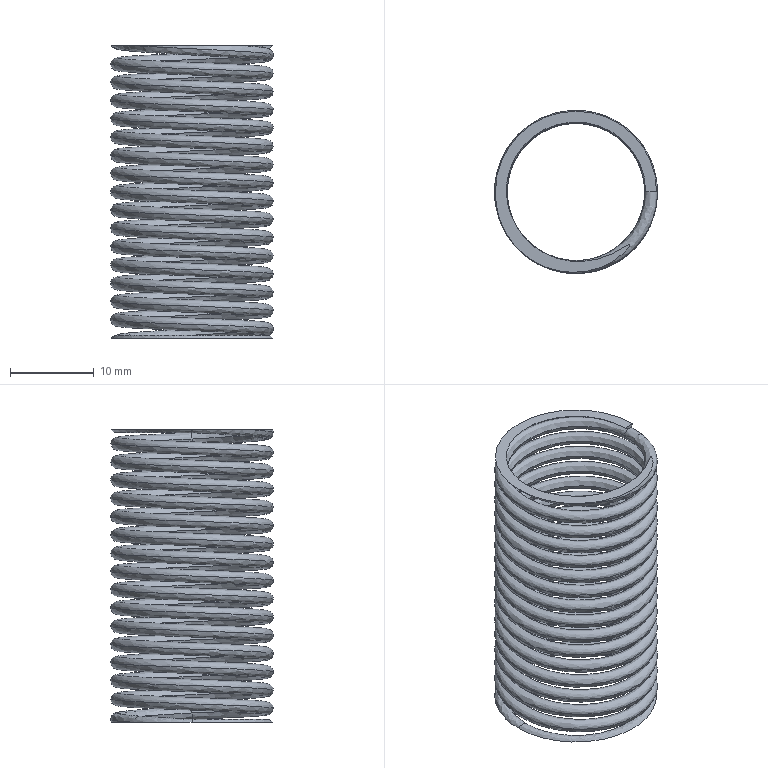Part | SolidWorks | features Helix 3, Cut 2, CompositeCurve 1, Sweep 1 | 1 solid | 12 faces | box 19.5 x 19.5 x 35.05 mm | volume 1610 mm3 | spline 8 | plane 4